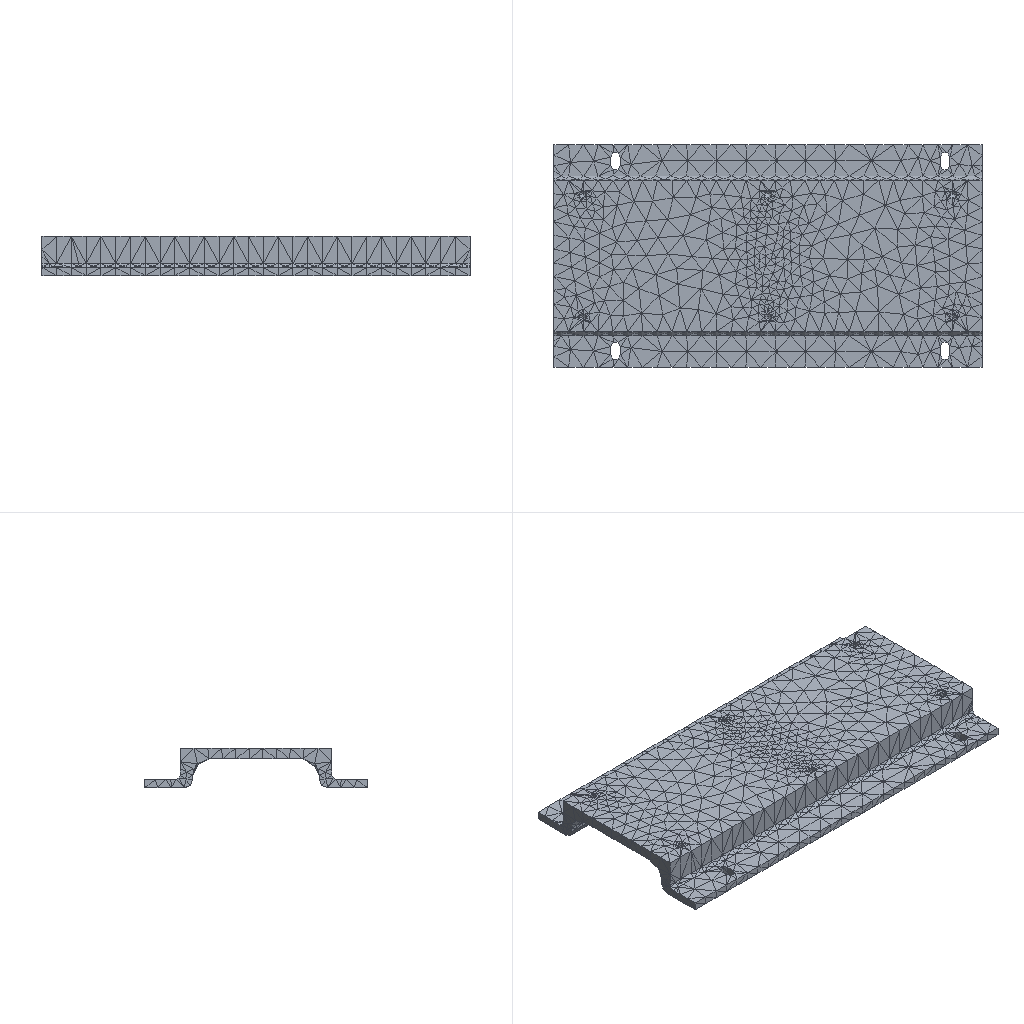Simulation study | ansys workbench
Set-up summary:
category,name,step,type,value,unit,region
solver,ansys_workbench
units,SI m-kg-s (Pa),,stated,"/units,MKS"
analysis,LS1,,static
load_step,LS1,LS1,static,nsubst=1; time=1
mesh,nodes,,,11601
mesh,elements,,,7068
element_type,SOLID187,,,6262
element_type,CONTA174,,,806
material,Structural Steel,,E,2e+11,Pa
material,Structural Steel,,nu,0.3
material,Structural Steel,,density,7850,kg m^-3
material,Structural Steel,,conductivity,60.5,W m^-1 C^-1
material,Structural Steel,,specific_heat,434,J kg^-1 C^-1
material,Structural Steel,,cte,1.2e-05,C^-1
material,Structural Steel,,permeability,10000
material,Structural Steel,,resistivity,1.7e-07,kg m^3 A^-2 s^-3
load,,LS1,moment,"1000 [dir=(0, 0, 1) n=3]",,all
bc,Fixed Supports,model,fixed,[dofs=ALL],,_FIXEDSU
contact,contact 1,,bonded (always),element=CONTA174
named_set,_FIXEDSU,,node,654
Ansys APDL input file, long lists of numbers shortened:
/batch
/config,noeldb,1     ! force off writing results to database
*get,_wallstrt,active,,time,wall
! ANSYS input file written by Workbench version 2024 R1
! File used for geometry attach:
/title,wbnew--____ (A5)
! ****** Begin Custom Load Command Snippet ******
/COM, ACT Extensions:
/COM,     LSDYNA, 2024.1
/COM,/COM,     ANSYSMotion, 2024.1
/COM,
! ****** End   Custom Load Command Snippet ******
*DIM,_wb_ProjectScratch_dir,string,248
_wb_ProjectScratch_dir(1) = ''
*DIM,_wb_SolverFiles_dir,string,248
_wb_SolverFiles_dir(1) = ''
*DIM,_wb_userfiles_dir,string,248
_wb_userfiles_dir(1) = ''
/com,--- Data in consistent MKS units. See Solving Units in the help system for more information.
/units,MKS
/nopr
/wb,file,start              !  signify a WB generated input file
/prep7
! Turn off shape checking because checks already performed inside WB mesher.
! See help system for more information.
SHPP,OFF,,NOWARN
/nolist
etcon,set             ! allow ANSYS to choose best KEYOP's for 180x elements, resets any applicable keyopt to MAPDL defaults
/com,*********** Nodes for the whole assembly ***********
nblock,3,,12760
(1i9,3e20.9e3)
        1     4.930000000E-01    -4.500000000E-02    -9.000000000E-02
! (11599 more lines like these left out)
-1
/com,*********** Nodes for all Remote Points ***********
nblock,3
(1i9,3e20.9e3)
    11601     2.329999927E-01     9.000000000E-02    -4.200000000E-02
-1
/wb,elem,start            !  set before creation of elements
/com,*********** Elements for Body 1 "______" ***********
et,1,187
eblock,19,solid,,6262
(19i9)
        1        1        1        1        0        0        0        0       10        0        1     1582     1700     1887     1884    10865    11345    10869    10868
! (12523 more lines like these left out)
-1
/wb,elem,end               !  done creating elements
/com,*********** Send User Defined Coordinate System(s) ***********
csys,0
toffst,273.15,  ! Temperature offset from absolute zero
/com,*********** Set Reference Temperature ***********
tref,22.
/wb,mat,start              !  starting to send materials
/com,*********** Send Materials ***********
Temperature = 'TEMP' ! Temperature
MP,DENS,1,7850,	! kg m^-3
MP,ALPX,1,1.2e-05,	! C^-1
MP,C,1,434,	! J kg^-1 C^-1
MP,KXX,1,60.5,	! W m^-1 C^-1
MP,RSVX,1,1.7e-07,	! kg m^3 A^-2 s^-3
MP,EX,1,200000000000,	! Pa
MP,NUXY,1,0.3,
MP,MURX,1,10000,
/wb,mat,end                !  done sending materials
!************************* Model Summary ********************
!åç®±ä½è¿æ¥æ¿,	ç»æé¢,	matid,	1
!************************* End Model Summary ********************
! get the diagonal of the bounding box. Needed later for other things
*get,_xmin,node,,mnloc,x
*get,_ymin,node,,mnloc,y
*get,_zmin,node,,mnloc,z
*get,_xmax,node,,mxloc,x
*get,_ymax,node,,mxloc,y
*get,_zmax,node,,mxloc,z
_ASMDIAG=(_xmax-_xmin)*(_xmax-_xmin)+(_ymax-_ymin)*(_ymax-_ymin)+(_zmax-_zmin)*(_zmax-_zmin)
_ASMDIAG=SQRT(_ASMDIAG)
/wb,contact,start          !  starting to send contact
/wb,contact,end            !  done creating contacts
/golist
/wb,load,start             !  starting to send loads
/com,*********** Fixed Supports ***********
CMBLOCK,_FIXEDSU,NODE,      654
(8i10)
         1        32        33        34        35        36        37        38
! (81 more lines like these left out)
cmsel,s,_FIXEDSU
d,all,all
nsel,all
/com,*********** Create Remote Point "ÄÚ²¿Ô¶³Ìµã" ***********
! -------- Remote Point Used by "Á¦¾Ø" --------
*set,tid,3
*set,cid,2
et,cid,174
et,tid,170
keyo,tid,2,1               ! Don't fix the pilot node
keyo,tid,4,111111
keyo,cid,12,5              ! Bonded Contact
keyo,cid,4,1               ! Deformable RBE3 style load
keyo,cid,2,2               ! MPC style contact
eblock,10,,,806
(15i9)
     9366        2        2        2        0     1122     1379     1229     1229     9055     9725     1229     9052
! (805 more lines like these left out)
-1
*set,_npilot,11601
_npilot31=_npilot
type,tid
mat ,cid
real,cid
tshape,pilo
en,10172,_npilot
tshape
/com,*********** Construct Moment Using Remote Attachment ***********
/gst,on,on
fini
*get,_numnode,node,0,count
*get,_numelem,elem,0,count
*get, _MAXELEMNUM, elem, 0, NUM, MAX
*get, _MAXNODENUM, node, 0, NUM, MAX
*get, _MAXELEMTYPE, etyp, 0, NUM, MAX
*get, _MAXREALCONST, rcon, 0, NUM, MAX
/go
/wb,load,end               !  done creating loads
/com,--- Number of total nodes = %_numnode%
/com,--- Number of contact elements = 806
/com,--- Number of spring elements = 0
/com,--- Number of bearing elements = 0
/com,--- Number of solid elements = 6262
/com,--- Number of condensed parts = 0
/com,--- Number of total elements = %_numelem%
*get,_wallbsol,active,,time,wall
/com,****************************************************************************
/com,*************************    SOLUTION       ********************************
/com,****************************************************************************
/solu
antype,0                   ! static analysis
_thickRatio=  0     ! Ratio of thick parts in the model
eqsl,sparse,,,,,1
cntr,print,1               ! print out contact info and also make no initial contact an error
cncheck,dmp		!	Enable program controlled contact splitting for distributed memory parallel run
dmpoption,emat,no             ! Don't combine emat file for DANSYS
dmpoption,esav,no             ! Don't combine esav file for DANSYS
nldiag,cont,iter           ! print out contact info each equilibrium iteration
rescontrol,,none                 ! Do not keep any restart files
/com,****************************************************
/com,******************* SOLVE FOR LS 1 OF 1 ****************
nsel,s,node,,11601
f,all,mx,0.
f,all,my,0.
f,all,mz,1000.
nsel,all
/nopr
/gopr
nsub,1,1,1
time,1.
outres,erase
outres,all,none
outres,nsol,all,
outres,rsol,all
outres,eangl,all
outres,etmp,all
outres,veng,all
outres,strs,all,
outres,epel,all,
outres,eppl,all,
outres,cont,all,
! *********** WB SOLVE COMMAND ***********
! check interactive state
*get,ANSINTER_,active,,int
*if,ANSINTER_,ne,0,then
/eof
*endif
solve
/com *************** Write FE CONNECTORS *********
CEWRITE,file,ce,,INTE
/com,****************************************************
/com,*************** FINISHED SOLVE FOR LS 1 *************
*get,_wallasol,active,,time,wall
/nopr
*get,_numnode,node,0,count
*get,_numelem,elem,0,count
*get, _MAXELEMNUM, elem, 0, NUM, MAX
*get, _MAXNODENUM, node, 0, NUM, MAX,,,INTERNAL
*get, _MAXELEMTYPE, etyp, 0, NUM, MAX
*get, _MAXREALCONST, rcon, 0, NUM, MAX
*get,_NSOLTHREADS,active,0,ntfs
*get,_NSOLPROCESSES,active,0,npfs
/gopr
/post1
xmlo,ENCODING,ISO-8859-1
xmlo,parm
/xml,parm,xml
fini
/gopr
*get,_walldone,active,,time,wall
_preptime=(_wallbsol-_wallstrt)*3600
_solvtime=(_wallasol-_wallbsol)*3600
_posttime=(_walldone-_wallasol)*3600
_totaltim=(_walldone-_wallstrt)*3600
*get,_dlbratio,active,0,solu,dlbr
*get,_combtime,active,0,solu,comb
*get,_ssmode,active,0,solu,ssmm
*get,_ndofs,active,0,solu,ndof
*get,_sol_end_time,active,0,set,time
*if,_sol_end_time,eq,1.,then
/fclean				!clean distributed files
*endif
/com,--- Total number of nodes = %_numnode%
/com,--- Total number of elements = %_numelem%
/com,--- Element load balance ratio = %_dlbratio%
/com,--- Time to combine distributed files = %_combtime%
/com,--- Sparse memory mode = %_ssmode%
/com,--- Number of DOF = %_ndofs%
/wb,file,end               ! done with WB generated input
Results summary:
result,analyses[0].index,,,1
result,analyses[0].system,,,SYS
result,analyses[0].deck,,,deck.dat
result,analyses[0].solve_status,,,completed
result,analyses[0].analysis_type,,,static
result,analyses[0].physics,,,mechanical
result,analyses[0].unit_system,,,"MKS: m, kg, N, s, V, A, degC"
result,analyses[0].n_sets,,,1
result,analyses[0].load_steps[0].set,set=1,,1
result,analyses[0].load_steps[0].time_or_freq,set=1,,1
result,analyses[0].load_steps[0].max_displacement_magnitude,set=1,,1.66369e-06
result,analyses[0].load_steps[0].max_von_mises_nodal,set=1,,4.44036e+06
result,analyses[0].load_steps[0].reaction_force_sum_xyz[1],set=1,,-1.82106e-08
result,analyses[0].load_steps[0].reaction_force_sum_xyz[2],set=1,,1.27465e-05
result,analyses[0].load_steps[0].reaction_force_sum_xyz[3],set=1,,-1.28454e-09
result,geometry_export[0][0],,,.step
result,geometry_export[0][1],,,ok
result,geometry_export[0][2],,,1